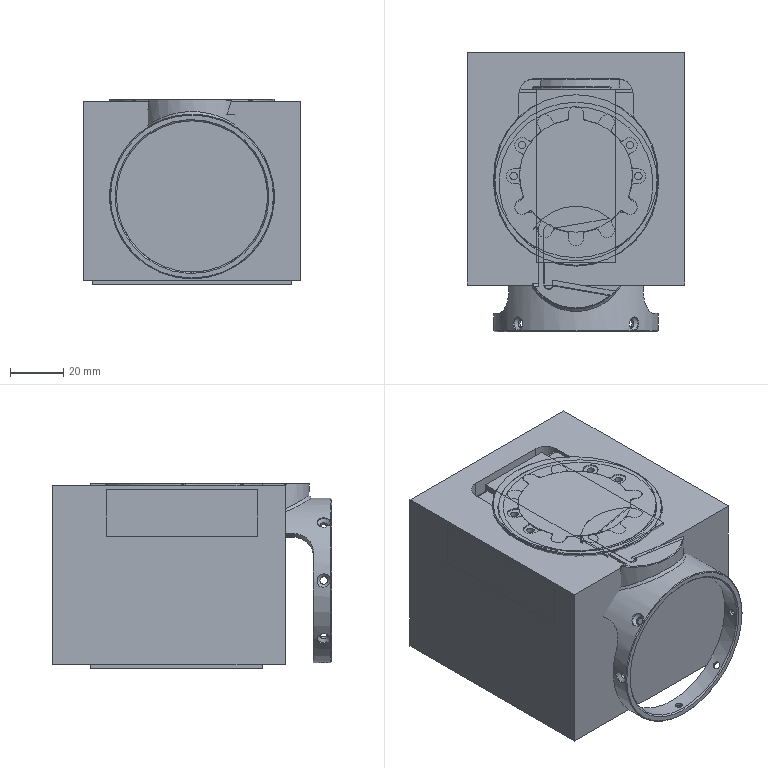NC program | NX | posted with a generic post | part box 82 x 105.2 x 70 mm
Whole program, first 1625 of 1919 lines:
N10 G17 G21 G94 G90
(轮廓开粗_2 , TOOL : 粗刀D10)
N12 T15 M6
N14 G53
N16 G17 G0 G90 X-36.218 Y-6.536 B0. C0. S7000 M3
N18 G43 Z10. H15
N20 Z2.07
N22 G94 G1 Z0.07 F2500.
N24 G41 X-32.352 Y-1.928 D15
N26 G3 X-31.65 Y0. R3.
N28 G2 X0. Y31.65 R31.65
N30 X-31.65 Y0. R-31.65
N32 G3 X-32.352 Y1.928 R3.
N34 G40
N36 G1 X-32.48 Y2.082
N38 X-29.48 Y-2.082
N40 G41 X-29.352 Y-1.928
N42 G3 X-28.65 Y0. R3.
N44 G2 X0. Y28.65 R28.65
N46 X-28.65 Y0. R-28.65
N48 G3 X-29.352 Y1.928 R3.
N50 G40
N52 G1 X-29.48 Y2.082
N54 X-26.48 Y-2.082
N56 G41 X-26.352 Y-1.928
N58 G3 X-25.65 Y0. R3.
N60 G2 X0. Y25.65 R25.65
N62 X-25.65 Y0. R-25.65
N64 G3 X-26.352 Y1.928 R3.
N66 G40
N68 G1 X-26.48 Y2.082
N70 X-23.48 Y-2.082
N72 G41 X-23.352 Y-1.928
N74 G3 X-22.65 Y0. R3.
N76 G2 X0. Y22.65 R22.65
N78 X-22.65 Y0. R-22.65
N80 G3 X-23.352 Y1.928 R3.
N82 G1 X-29.295 Y9.011
N84 G40
N86 X-29.424 Y9.165
N88 Z2.07
N90 G0 Z10.
(轮廓开粗_2_COPY , TOOL : 粗刀D10)
N92 X-1.314 Y-12.785 S5500
N94 Z-1.5
N96 G1 Z-3.5 F1500.
N98 G41 X-1.241 Y-14.137
N100 G3 X0.864 Y-16.027 R2.
N102 X16.027 Y0.864 R16.05
N104 X0.864 Y-16.027 R-16.05
N106 X2.753 Y-13.922 R2.
N108 G1 X2.691 Y-12.769
N110 G40
N112 X2.68 Y-12.57
N114 Z-1.5
N116 G0 Z10.
N118 M5
(中心孔 , TOOL : 中心钻D6)
N120 T01 M6
N122 G53
N124 G17 G0 G90 X-11.75 Y20.352 B0. C0. S2000 M3
N126 G43 Z10. H1
N128 G94 G81 G98 Z-1.5 F180. R1.
N130 X-20.352 Y11.75
N132 X-23.5 Y0.
N134 X-11.75 Y-20.352
N136 X0. Y-23.5
N138 X11.75 Y-20.352
N140 X23.5 Y0.
N142 X20.352 Y11.75
N144 X11.75 Y20.352
N146 G80
N148 G0 X11.75 Y20.352 Z10.
N150 M5
(钻头D2.9- , TOOL : 钻头D2.8)
N152 T17 M6
N154 G53
N156 G17 G0 G90 X-20.352 Y11.75 B0. C0. S2500 M3
N158 G43 Z10. H17
N160 G94 G83 G98 Z-5.341 F200. Q3. R1.
N162 X-11.75 Y20.352
N164 X11.75
N166 X20.352 Y11.75
N168 X23.5 Y0.
N170 X11.75 Y-20.352
N172 X0. Y-23.5
N174 X-11.75 Y-20.352
N176 X-23.5 Y0.
N178 G80
N180 G0 X-23.5 Y0. Z10.
N182 M5
(轮廓开粗_3 , TOOL : 粗刀D4)
N184 T18 M6
N186 G53
N188 G17 G0 G90 X4.767 Y17.977 B0. C0. S8500 M3
N190 G43 Z10. H18
N192 Z-0.329
N194 G41 G94 G1 X4.484 Y18.337 F2000. D18
N196 G3 X3.902 Y18.697 R1.
N198 G2 X0.6 Y22.76 R4.15
N200 G1 Y23.5
N202 G3 X0. Y24.1 R0.6
N204 X-0.6 Y23.5 R0.6
N206 G1 Y22.76
N208 G2 X-3.902 Y18.697 R4.15
N210 G3 X-4.484 Y18.337 R1.
N212 G1 X-4.643 Y18.134
N214 G40
N216 X-4.767 Y17.977
N218 G0 X4.767 Z-0.657
N220 G41 G1 X4.484 Y18.337
N222 G3 X3.902 Y18.697 R1.
N224 G2 X0.6 Y22.76 R4.15
N226 G1 Y23.5
N228 G3 X0. Y24.1 R0.6
N230 X-0.6 Y23.5 R0.6
N232 G1 Y22.76
N234 G2 X-3.902 Y18.697 R4.15
N236 G3 X-4.484 Y18.337 R1.
N238 G1 X-4.643 Y18.134
N240 G40
N242 X-4.767 Y17.977
N244 G0 X4.767 Z-0.986
N246 G41 G1 X4.484 Y18.337
N248 G3 X3.902 Y18.697 R1.
N250 G2 X0.6 Y22.76 R4.15
N252 G1 Y23.5
N254 G3 X0. Y24.1 R0.6
N256 X-0.6 Y23.5 R0.6
N258 G1 Y22.76
N260 G2 X-3.902 Y18.697 R4.15
N262 G3 X-4.484 Y18.337 R1.
N264 G1 X-4.643 Y18.134
N266 G40
N268 X-4.767 Y17.977
N270 G0 X4.767 Z-1.315
N272 G41 G1 X4.484 Y18.337
N274 G3 X3.902 Y18.697 R1.
N276 G2 X0.6 Y22.76 R4.15
N278 G1 Y23.5
N280 G3 X0. Y24.1 R0.6
N282 X-0.6 Y23.5 R0.6
N284 G1 Y22.76
N286 G2 X-3.902 Y18.697 R4.15
N288 G3 X-4.484 Y18.337 R1.
N290 G1 X-4.643 Y18.134
N292 G40
N294 X-4.767 Y17.977
N296 G0 X4.767 Z-1.643
N298 G41 G1 X4.484 Y18.337
N300 G3 X3.902 Y18.697 R1.
N302 G2 X0.6 Y22.76 R4.15
N304 G1 Y23.5
N306 G3 X0. Y24.1 R0.6
N308 X-0.6 Y23.5 R0.6
N310 G1 Y22.76
N312 G2 X-3.902 Y18.697 R4.15
N314 G3 X-4.484 Y18.337 R1.
N316 G1 X-4.643 Y18.134
N318 G40
N320 X-4.767 Y17.977
N322 G0 X4.767 Z-1.972
N324 G41 G1 X4.484 Y18.337
N326 G3 X3.902 Y18.697 R1.
N328 G2 X0.6 Y22.76 R4.15
N330 G1 Y23.5
N332 G3 X0. Y24.1 R0.6
N334 X-0.6 Y23.5 R0.6
N336 G1 Y22.76
N338 G2 X-3.902 Y18.697 R4.15
N340 G3 X-4.484 Y18.337 R1.
N342 G1 X-4.643 Y18.134
N344 G40
N346 X-4.767 Y17.977
N348 G0 X4.767 Z-2.301
N350 G41 G1 X4.484 Y18.337
N352 G3 X3.902 Y18.697 R1.
N354 G2 X0.6 Y22.76 R4.15
N356 G1 Y23.5
N358 G3 X0. Y24.1 R0.6
N360 X-0.6 Y23.5 R0.6
N362 G1 Y22.76
N364 G2 X-3.902 Y18.697 R4.15
N366 G3 X-4.484 Y18.337 R1.
N368 G1 X-4.643 Y18.134
N370 G40
N372 X-4.767 Y17.977
N374 G0 X4.767 Z-2.629
N376 G41 G1 X4.484 Y18.337
N378 G3 X3.902 Y18.697 R1.
N380 G2 X0.6 Y22.76 R4.15
N382 G1 Y23.5
N384 G3 X0. Y24.1 R0.6
N386 X-0.6 Y23.5 R0.6
N388 G1 Y22.76
N390 G2 X-3.902 Y18.697 R4.15
N392 G3 X-4.484 Y18.337 R1.
N394 G1 X-4.643 Y18.134
N396 G40
N398 X-4.767 Y17.977
N400 G0 X4.767 Z-2.958
N402 G41 G1 X4.484 Y18.337
N404 G3 X3.902 Y18.697 R1.
N406 G2 X0.6 Y22.76 R4.15
N408 G1 Y23.5
N410 G3 X0. Y24.1 R0.6
N412 X-0.6 Y23.5 R0.6
N414 G1 Y22.76
N416 G2 X-3.902 Y18.697 R4.15
N418 G3 X-4.484 Y18.337 R1.
N420 G1 X-4.643 Y18.134
N422 G40
N424 X-4.767 Y17.977
N426 G0 X4.767 Z-3.287
N428 G41 G1 X4.484 Y18.337
N430 G3 X3.902 Y18.697 R1.
N432 G2 X0.6 Y22.76 R4.15
N434 G1 Y23.5
N436 G3 X0. Y24.1 R0.6
N438 X-0.6 Y23.5 R0.6
N440 G1 Y22.76
N442 G2 X-3.902 Y18.697 R4.15
N444 G3 X-4.484 Y18.337 R1.
N446 G1 X-4.643 Y18.134
N448 G40
N450 X-4.767 Y17.977
N452 G0 X4.767 Z-3.615
N454 G41 G1 X4.484 Y18.337
N456 G3 X3.902 Y18.697 R1.
N458 G2 X0.6 Y22.76 R4.15
N460 G1 Y23.5
N462 G3 X0. Y24.1 R0.6
N464 X-0.6 Y23.5 R0.6
N466 G1 Y22.76
N468 G2 X-3.902 Y18.697 R4.15
N470 G3 X-4.484 Y18.337 R1.
N472 G1 X-4.643 Y18.134
N474 G40
N476 X-4.767 Y17.977
N478 G0 X4.767 Z-3.944
N480 G41 G1 X4.484 Y18.337
N482 G3 X3.902 Y18.697 R1.
N484 G2 X0.6 Y22.76 R4.15
N486 G1 Y23.5
N488 G3 X0. Y24.1 R0.6
N490 X-0.6 Y23.5 R0.6
N492 G1 Y22.76
N494 G2 X-3.902 Y18.697 R4.15
N496 G3 X-4.484 Y18.337 R1.
N498 G1 X-4.643 Y18.134
N500 G40
N502 X-4.767 Y17.977
N504 G0 X4.767 Z-4.273
N506 G41 G1 X4.484 Y18.337
N508 G3 X3.902 Y18.697 R1.
N510 G2 X0.6 Y22.76 R4.15
N512 G1 Y23.5
N514 G3 X0. Y24.1 R0.6
N516 X-0.6 Y23.5 R0.6
N518 G1 Y22.76
N520 G2 X-3.902 Y18.697 R4.15
N522 G3 X-4.484 Y18.337 R1.
N524 G1 X-4.643 Y18.134
N526 G40
N528 X-4.767 Y17.977
N530 G0 X4.767 Z-4.601
N532 G41 G1 X4.484 Y18.337
N534 G3 X3.902 Y18.697 R1.
N536 G2 X0.6 Y22.76 R4.15
N538 G1 Y23.5
N540 G3 X0. Y24.1 R0.6
N542 X-0.6 Y23.5 R0.6
N544 G1 Y22.76
N546 G2 X-3.902 Y18.697 R4.15
N548 G3 X-4.484 Y18.337 R1.
N550 G1 X-4.643 Y18.134
N552 G40
N554 X-4.767 Y17.977
N556 G0 X4.767 Z-4.93
N558 G41 G1 X4.484 Y18.337
N560 G3 X3.902 Y18.697 R1.
N562 G2 X0.6 Y22.76 R4.15
N564 G1 Y23.5
N566 G3 X0. Y24.1 R0.6
N568 X-0.6 Y23.5 R0.6
N570 G1 Y22.76
N572 G2 X-3.902 Y18.697 R4.15
N574 G3 X-4.484 Y18.337 R1.
N576 G1 X-4.643 Y18.134
N578 G40
N580 X-4.767 Y17.977
N582 G0 Z10.
N584 X-17.952 Y-4.86
N586 Z-0.329
N588 G41 G1 X-18.122 Y-5.286
N590 G3 X-18.143 Y-5.969 R1.
N592 G2 X-20.01 Y-10.86 R4.15
N594 G1 X-20.652 Y-11.23
N596 G3 X-20.871 Y-12.05 R0.6
N598 X-20.052 Y-12.27 R0.6
N600 G1 X-19.41 Y-11.899
N602 G2 X-14.241 Y-12.728 R4.15
N604 G3 X-13.638 Y-13.051 R1.
N606 G1 X-13.383 Y-13.088
N608 G40
N610 X-13.185 Y-13.117
N612 G0 X-17.952 Y-4.86 Z-0.657
N614 G41 G1 X-18.122 Y-5.286
N616 G3 X-18.143 Y-5.969 R1.
N618 G2 X-20.01 Y-10.86 R4.15
N620 G1 X-20.652 Y-11.23
N622 G3 X-20.871 Y-12.05 R0.6
N624 X-20.052 Y-12.27 R0.6
N626 G1 X-19.41 Y-11.899
N628 G2 X-14.241 Y-12.728 R4.15
N630 G3 X-13.638 Y-13.051 R1.
N632 G1 X-13.383 Y-13.088
N634 G40
N636 X-13.185 Y-13.117
N638 G0 X-17.952 Y-4.86 Z-0.986
N640 G41 G1 X-18.122 Y-5.286
N642 G3 X-18.143 Y-5.969 R1.
N644 G2 X-20.01 Y-10.86 R4.15
N646 G1 X-20.652 Y-11.23
N648 G3 X-20.871 Y-12.05 R0.6
N650 X-20.052 Y-12.27 R0.6
N652 G1 X-19.41 Y-11.899
N654 G2 X-14.241 Y-12.728 R4.15
N656 G3 X-13.638 Y-13.051 R1.
N658 G1 X-13.383 Y-13.088
N660 G40
N662 X-13.185 Y-13.117
N664 G0 X-17.952 Y-4.86 Z-1.315
N666 G41 G1 X-18.122 Y-5.286
N668 G3 X-18.143 Y-5.969 R1.
N670 G2 X-20.01 Y-10.86 R4.15
N672 G1 X-20.652 Y-11.23
N674 G3 X-20.871 Y-12.05 R0.6
N676 X-20.052 Y-12.27 R0.6
N678 G1 X-19.41 Y-11.899
N680 G2 X-14.241 Y-12.728 R4.15
N682 G3 X-13.638 Y-13.051 R1.
N684 G1 X-13.383 Y-13.088
N686 G40
N688 X-13.185 Y-13.117
N690 G0 X-17.952 Y-4.86 Z-1.643
N692 G41 G1 X-18.122 Y-5.286
N694 G3 X-18.143 Y-5.969 R1.
N696 G2 X-20.01 Y-10.86 R4.15
N698 G1 X-20.652 Y-11.23
N700 G3 X-20.871 Y-12.05 R0.6
N702 X-20.052 Y-12.27 R0.6
N704 G1 X-19.41 Y-11.899
N706 G2 X-14.241 Y-12.728 R4.15
N708 G3 X-13.638 Y-13.051 R1.
N710 G1 X-13.383 Y-13.088
N712 G40
N714 X-13.185 Y-13.117
N716 G0 X-17.952 Y-4.86 Z-1.972
N718 G41 G1 X-18.122 Y-5.286
N720 G3 X-18.143 Y-5.969 R1.
N722 G2 X-20.01 Y-10.86 R4.15
N724 G1 X-20.652 Y-11.23
N726 G3 X-20.871 Y-12.05 R0.6
N728 X-20.052 Y-12.27 R0.6
N730 G1 X-19.41 Y-11.899
N732 G2 X-14.241 Y-12.728 R4.15
N734 G3 X-13.638 Y-13.051 R1.
N736 G1 X-13.383 Y-13.088
N738 G40
N740 X-13.185 Y-13.117
N742 G0 X-17.952 Y-4.86 Z-2.301
N744 G41 G1 X-18.122 Y-5.286
N746 G3 X-18.143 Y-5.969 R1.
N748 G2 X-20.01 Y-10.86 R4.15
N750 G1 X-20.652 Y-11.23
N752 G3 X-20.871 Y-12.05 R0.6
N754 X-20.052 Y-12.27 R0.6
N756 G1 X-19.41 Y-11.899
N758 G2 X-14.241 Y-12.728 R4.15
N760 G3 X-13.638 Y-13.051 R1.
N762 G1 X-13.383 Y-13.088
N764 G40
N766 X-13.185 Y-13.117
N768 G0 X-17.952 Y-4.86 Z-2.629
N770 G41 G1 X-18.122 Y-5.286
N772 G3 X-18.143 Y-5.969 R1.
N774 G2 X-20.01 Y-10.86 R4.15
N776 G1 X-20.652 Y-11.23
N778 G3 X-20.871 Y-12.05 R0.6
N780 X-20.052 Y-12.27 R0.6
N782 G1 X-19.41 Y-11.899
N784 G2 X-14.241 Y-12.728 R4.15
N786 G3 X-13.638 Y-13.051 R1.
N788 G1 X-13.383 Y-13.088
N790 G40
N792 X-13.185 Y-13.117
N794 G0 X-17.952 Y-4.86 Z-2.958
N796 G41 G1 X-18.122 Y-5.286
N798 G3 X-18.143 Y-5.969 R1.
N800 G2 X-20.01 Y-10.86 R4.15
N802 G1 X-20.652 Y-11.23
N804 G3 X-20.871 Y-12.05 R0.6
N806 X-20.052 Y-12.27 R0.6
N808 G1 X-19.41 Y-11.899
N810 G2 X-14.241 Y-12.728 R4.15
N812 G3 X-13.638 Y-13.051 R1.
N814 G1 X-13.383 Y-13.088
N816 G40
N818 X-13.185 Y-13.117
N820 G0 X-17.952 Y-4.86 Z-3.287
N822 G41 G1 X-18.122 Y-5.286
N824 G3 X-18.143 Y-5.969 R1.
N826 G2 X-20.01 Y-10.86 R4.15
N828 G1 X-20.652 Y-11.23
N830 G3 X-20.871 Y-12.05 R0.6
N832 X-20.052 Y-12.27 R0.6
N834 G1 X-19.41 Y-11.899
N836 G2 X-14.241 Y-12.728 R4.15
N838 G3 X-13.638 Y-13.051 R1.
N840 G1 X-13.383 Y-13.088
N842 G40
N844 X-13.185 Y-13.117
N846 G0 X-17.952 Y-4.86 Z-3.615
N848 G41 G1 X-18.122 Y-5.286
N850 G3 X-18.143 Y-5.969 R1.
N852 G2 X-20.01 Y-10.86 R4.15
N854 G1 X-20.652 Y-11.23
N856 G3 X-20.871 Y-12.05 R0.6
N858 X-20.052 Y-12.27 R0.6
N860 G1 X-19.41 Y-11.899
N862 G2 X-14.241 Y-12.728 R4.15
N864 G3 X-13.638 Y-13.051 R1.
N866 G1 X-13.383 Y-13.088
N868 G40
N870 X-13.185 Y-13.117
N872 G0 X-17.952 Y-4.86 Z-3.944
N874 G41 G1 X-18.122 Y-5.286
N876 G3 X-18.143 Y-5.969 R1.
N878 G2 X-20.01 Y-10.86 R4.15
N880 G1 X-20.652 Y-11.23
N882 G3 X-20.871 Y-12.05 R0.6
N884 X-20.052 Y-12.27 R0.6
N886 G1 X-19.41 Y-11.899
N888 G2 X-14.241 Y-12.728 R4.15
N890 G3 X-13.638 Y-13.051 R1.
N892 G1 X-13.383 Y-13.088
N894 G40
N896 X-13.185 Y-13.117
N898 G0 X-17.952 Y-4.86 Z-4.273
N900 G41 G1 X-18.122 Y-5.286
N902 G3 X-18.143 Y-5.969 R1.
N904 G2 X-20.01 Y-10.86 R4.15
N906 G1 X-20.652 Y-11.23
N908 G3 X-20.871 Y-12.05 R0.6
N910 X-20.052 Y-12.27 R0.6
N912 G1 X-19.41 Y-11.899
N914 G2 X-14.241 Y-12.728 R4.15
N916 G3 X-13.638 Y-13.051 R1.
N918 G1 X-13.383 Y-13.088
N920 G40
N922 X-13.185 Y-13.117
N924 G0 X-17.952 Y-4.86 Z-4.601
N926 G41 G1 X-18.122 Y-5.286
N928 G3 X-18.143 Y-5.969 R1.
N930 G2 X-20.01 Y-10.86 R4.15
N932 G1 X-20.652 Y-11.23
N934 G3 X-20.871 Y-12.05 R0.6
N936 X-20.052 Y-12.27 R0.6
N938 G1 X-19.41 Y-11.899
N940 G2 X-14.241 Y-12.728 R4.15
N942 G3 X-13.638 Y-13.051 R1.
N944 G1 X-13.383 Y-13.088
N946 G40
N948 X-13.185 Y-13.117
N950 G0 X-17.952 Y-4.86 Z-4.93
N952 G41 G1 X-18.122 Y-5.286
N954 G3 X-18.143 Y-5.969 R1.
N956 G2 X-20.01 Y-10.86 R4.15
N958 G1 X-20.652 Y-11.23
N960 G3 X-20.871 Y-12.05 R0.6
N962 X-20.052 Y-12.27 R0.6
N964 G1 X-19.41 Y-11.899
N966 G2 X-14.241 Y-12.728 R4.15
N968 G3 X-13.638 Y-13.051 R1.
N970 G1 X-13.383 Y-13.088
N972 G40
N974 X-13.185 Y-13.117
N976 G0 Z10.
N978 X13.185
N980 Z-0.329
N982 G41 G1 X13.638 Y-13.051
N984 G3 X14.241 Y-12.728 R1.
N986 G2 X19.41 Y-11.899 R4.15
N988 G1 X20.052 Y-12.27
N990 G3 X20.871 Y-12.05 R0.6
N992 X20.652 Y-11.23 R0.6
N994 G1 X20.01 Y-10.86
N996 G2 X18.143 Y-5.969 R4.15
N998 G3 X18.122 Y-5.286 R1.
N1000 G1 X18.026 Y-5.046
N1002 G40
N1004 X17.952 Y-4.86
N1006 G0 X13.185 Y-13.117 Z-0.657
N1008 G41 G1 X13.638 Y-13.051
N1010 G3 X14.241 Y-12.728 R1.
N1012 G2 X19.41 Y-11.899 R4.15
N1014 G1 X20.052 Y-12.27
N1016 G3 X20.871 Y-12.05 R0.6
N1018 X20.652 Y-11.23 R0.6
N1020 G1 X20.01 Y-10.86
N1022 G2 X18.143 Y-5.969 R4.15
N1024 G3 X18.122 Y-5.286 R1.
N1026 G1 X18.026 Y-5.046
N1028 G40
N1030 X17.952 Y-4.86
N1032 G0 X13.185 Y-13.117 Z-0.986
N1034 G41 G1 X13.638 Y-13.051
N1036 G3 X14.241 Y-12.728 R1.
N1038 G2 X19.41 Y-11.899 R4.15
N1040 G1 X20.052 Y-12.27
N1042 G3 X20.871 Y-12.05 R0.6
N1044 X20.652 Y-11.23 R0.6
N1046 G1 X20.01 Y-10.86
N1048 G2 X18.143 Y-5.969 R4.15
N1050 G3 X18.122 Y-5.286 R1.
N1052 G1 X18.026 Y-5.046
N1054 G40
N1056 X17.952 Y-4.86
N1058 G0 X13.185 Y-13.117 Z-1.315
N1060 G41 G1 X13.638 Y-13.051
N1062 G3 X14.241 Y-12.728 R1.
N1064 G2 X19.41 Y-11.899 R4.15
N1066 G1 X20.052 Y-12.27
N1068 G3 X20.871 Y-12.05 R0.6
N1070 X20.652 Y-11.23 R0.6
N1072 G1 X20.01 Y-10.86
N1074 G2 X18.143 Y-5.969 R4.15
N1076 G3 X18.122 Y-5.286 R1.
N1078 G1 X18.026 Y-5.046
N1080 G40
N1082 X17.952 Y-4.86
N1084 G0 X13.185 Y-13.117 Z-1.643
N1086 G41 G1 X13.638 Y-13.051
N1088 G3 X14.241 Y-12.728 R1.
N1090 G2 X19.41 Y-11.899 R4.15
N1092 G1 X20.052 Y-12.27
N1094 G3 X20.871 Y-12.05 R0.6
N1096 X20.652 Y-11.23 R0.6
N1098 G1 X20.01 Y-10.86
N1100 G2 X18.143 Y-5.969 R4.15
N1102 G3 X18.122 Y-5.286 R1.
N1104 G1 X18.026 Y-5.046
N1106 G40
N1108 X17.952 Y-4.86
N1110 G0 X13.185 Y-13.117 Z-1.972
N1112 G41 G1 X13.638 Y-13.051
N1114 G3 X14.241 Y-12.728 R1.
N1116 G2 X19.41 Y-11.899 R4.15
N1118 G1 X20.052 Y-12.27
N1120 G3 X20.871 Y-12.05 R0.6
N1122 X20.652 Y-11.23 R0.6
N1124 G1 X20.01 Y-10.86
N1126 G2 X18.143 Y-5.969 R4.15
N1128 G3 X18.122 Y-5.286 R1.
N1130 G1 X18.026 Y-5.046
N1132 G40
N1134 X17.952 Y-4.86
N1136 G0 X13.185 Y-13.117 Z-2.301
N1138 G41 G1 X13.638 Y-13.051
N1140 G3 X14.241 Y-12.728 R1.
N1142 G2 X19.41 Y-11.899 R4.15
N1144 G1 X20.052 Y-12.27
N1146 G3 X20.871 Y-12.05 R0.6
N1148 X20.652 Y-11.23 R0.6
N1150 G1 X20.01 Y-10.86
N1152 G2 X18.143 Y-5.969 R4.15
N1154 G3 X18.122 Y-5.286 R1.
N1156 G1 X18.026 Y-5.046
N1158 G40
N1160 X17.952 Y-4.86
N1162 G0 X13.185 Y-13.117 Z-2.629
N1164 G41 G1 X13.638 Y-13.051
N1166 G3 X14.241 Y-12.728 R1.
N1168 G2 X19.41 Y-11.899 R4.15
N1170 G1 X20.052 Y-12.27
N1172 G3 X20.871 Y-12.05 R0.6
N1174 X20.652 Y-11.23 R0.6
N1176 G1 X20.01 Y-10.86
N1178 G2 X18.143 Y-5.969 R4.15
N1180 G3 X18.122 Y-5.286 R1.
N1182 G1 X18.026 Y-5.046
N1184 G40
N1186 X17.952 Y-4.86
N1188 G0 X13.185 Y-13.117 Z-2.958
N1190 G41 G1 X13.638 Y-13.051
N1192 G3 X14.241 Y-12.728 R1.
N1194 G2 X19.41 Y-11.899 R4.15
N1196 G1 X20.052 Y-12.27
N1198 G3 X20.871 Y-12.05 R0.6
N1200 X20.652 Y-11.23 R0.6
N1202 G1 X20.01 Y-10.86
N1204 G2 X18.143 Y-5.969 R4.15
N1206 G3 X18.122 Y-5.286 R1.
N1208 G1 X18.026 Y-5.046
N1210 G40
N1212 X17.952 Y-4.86
N1214 G0 X13.185 Y-13.117 Z-3.287
N1216 G41 G1 X13.638 Y-13.051
N1218 G3 X14.241 Y-12.728 R1.
N1220 G2 X19.41 Y-11.899 R4.15
N1222 G1 X20.052 Y-12.27
N1224 G3 X20.871 Y-12.05 R0.6
N1226 X20.652 Y-11.23 R0.6
N1228 G1 X20.01 Y-10.86
N1230 G2 X18.143 Y-5.969 R4.15
N1232 G3 X18.122 Y-5.286 R1.
N1234 G1 X18.026 Y-5.046
N1236 G40
N1238 X17.952 Y-4.86
N1240 G0 X13.185 Y-13.117 Z-3.615
N1242 G41 G1 X13.638 Y-13.051
N1244 G3 X14.241 Y-12.728 R1.
N1246 G2 X19.41 Y-11.899 R4.15
N1248 G1 X20.052 Y-12.27
N1250 G3 X20.871 Y-12.05 R0.6
N1252 X20.652 Y-11.23 R0.6
N1254 G1 X20.01 Y-10.86
N1256 G2 X18.143 Y-5.969 R4.15
N1258 G3 X18.122 Y-5.286 R1.
N1260 G1 X18.026 Y-5.046
N1262 G40
N1264 X17.952 Y-4.86
N1266 G0 X13.185 Y-13.117 Z-3.944
N1268 G41 G1 X13.638 Y-13.051
N1270 G3 X14.241 Y-12.728 R1.
N1272 G2 X19.41 Y-11.899 R4.15
N1274 G1 X20.052 Y-12.27
N1276 G3 X20.871 Y-12.05 R0.6
N1278 X20.652 Y-11.23 R0.6
N1280 G1 X20.01 Y-10.86
N1282 G2 X18.143 Y-5.969 R4.15
N1284 G3 X18.122 Y-5.286 R1.
N1286 G1 X18.026 Y-5.046
N1288 G40
N1290 X17.952 Y-4.86
N1292 G0 X13.185 Y-13.117 Z-4.273
N1294 G41 G1 X13.638 Y-13.051
N1296 G3 X14.241 Y-12.728 R1.
N1298 G2 X19.41 Y-11.899 R4.15
N1300 G1 X20.052 Y-12.27
N1302 G3 X20.871 Y-12.05 R0.6
N1304 X20.652 Y-11.23 R0.6
N1306 G1 X20.01 Y-10.86
N1308 G2 X18.143 Y-5.969 R4.15
N1310 G3 X18.122 Y-5.286 R1.
N1312 G1 X18.026 Y-5.046
N1314 G40
N1316 X17.952 Y-4.86
N1318 G0 X13.185 Y-13.117 Z-4.601
N1320 G41 G1 X13.638 Y-13.051
N1322 G3 X14.241 Y-12.728 R1.
N1324 G2 X19.41 Y-11.899 R4.15
N1326 G1 X20.052 Y-12.27
N1328 G3 X20.871 Y-12.05 R0.6
N1330 X20.652 Y-11.23 R0.6
N1332 G1 X20.01 Y-10.86
N1334 G2 X18.143 Y-5.969 R4.15
N1336 G3 X18.122 Y-5.286 R1.
N1338 G1 X18.026 Y-5.046
N1340 G40
N1342 X17.952 Y-4.86
N1344 G0 X13.185 Y-13.117 Z-4.93
N1346 G41 G1 X13.638 Y-13.051
N1348 G3 X14.241 Y-12.728 R1.
N1350 G2 X19.41 Y-11.899 R4.15
N1352 G1 X20.052 Y-12.27
N1354 G3 X20.871 Y-12.05 R0.6
N1356 X20.652 Y-11.23 R0.6
N1358 G1 X20.01 Y-10.86
N1360 G2 X18.143 Y-5.969 R4.15
N1362 G3 X18.122 Y-5.286 R1.
N1364 G1 X18.026 Y-5.046
N1366 G40
N1368 X17.952 Y-4.86
N1370 G0 Z10.
(轮廓开粗_3_COPY , TOOL : 粗刀D4)
N1372 X-17.728 Y5.559
N1374 Z-0.215
N1376 G41 G1 X-18.125 Y5.274
N1378 G3 X-18.511 Y4.708 R1.
N1380 X-18.827 Y3.219 R19.1
N1382 G2 X-21.932 Y0.6 R3.15
N1384 G1 X-23.5
N1386 G3 X-24.1 Y0. R0.6
N1388 X-23.5 Y-0.6 R0.6
N1390 G1 X-21.932
N1392 G2 X-18.827 Y-3.219 R3.15
N1394 G3 X-18.143 Y-5.969 R19.1
N1396 G2 X-20.01 Y-10.86 R4.15
N1398 G1 X-20.652 Y-11.23
N1400 G3 X-20.871 Y-12.05 R0.6
N1402 X-20.052 Y-12.27 R0.6
N1404 G1 X-19.41 Y-11.899
N1406 G2 X-14.241 Y-12.728 R4.15
N1408 G3 X-12.201 Y-14.695 R19.1
N1410 G2 X-11.485 Y-18.693 R3.15
N1412 G1 X-12.27 Y-20.052
N1414 G3 X-12.05 Y-20.871 R0.6
N1416 X-11.23 Y-20.652 R0.6
N1418 G1 X-10.446 Y-19.293
N1420 G2 X-6.626 Y-17.914 R3.15
N1422 G3 X-3.219 Y-18.827 R19.1
N1424 G2 X-0.6 Y-21.932 R3.15
N1426 G1 Y-23.5
N1428 G3 X0. Y-24.1 R0.6
N1430 X0.6 Y-23.5 R0.6
N1432 G1 Y-21.932
N1434 G2 X3.219 Y-18.827 R3.15
N1436 G3 X6.626 Y-17.914 R19.1
N1438 G2 X10.446 Y-19.293 R3.15
N1440 G1 X11.23 Y-20.652
N1442 G3 X12.05 Y-20.871 R0.6
N1444 X12.27 Y-20.052 R0.6
N1446 G1 X11.485 Y-18.693
N1448 G2 X12.201 Y-14.695 R3.15
N1450 G3 X14.241 Y-12.728 R19.1
N1452 G2 X19.41 Y-11.899 R4.15
N1454 G1 X20.052 Y-12.27
N1456 G3 X20.871 Y-12.05 R0.6
N1458 X20.652 Y-11.23 R0.6
N1460 G1 X20.01 Y-10.86
N1462 G2 X18.143 Y-5.969 R4.15
N1464 G3 X18.827 Y-3.219 R19.1
N1466 G2 X21.932 Y-0.6 R3.15
N1468 G1 X23.5
N1470 G3 X24.1 Y0. R0.6
N1472 X23.5 Y0.6 R0.6
N1474 G1 X21.932
N1476 G2 X18.827 Y3.219 R3.15
N1478 G3 X17.914 Y6.626 R19.1
N1480 G2 X19.293 Y10.446 R3.15
N1482 G1 X20.652 Y11.23
N1484 G3 X20.871 Y12.05 R0.6
N1486 X20.052 Y12.27 R0.6
N1488 G1 X18.693 Y11.485
N1490 G2 X14.695 Y12.201 R3.15
N1492 G3 X12.201 Y14.695 R19.1
N1494 G2 X11.485 Y18.693 R3.15
N1496 G1 X12.27 Y20.052
N1498 G3 X12.05 Y20.871 R0.6
N1500 X11.23 Y20.652 R0.6
N1502 G1 X10.446 Y19.293
N1504 G2 X6.626 Y17.914 R3.15
N1506 G3 X3.902 Y18.697 R19.1
N1508 G2 X0.6 Y22.76 R4.15
N1510 G1 Y23.5
N1512 G3 X0. Y24.1 R0.6
N1514 X-0.6 Y23.5 R0.6
N1516 G1 Y22.76
N1518 G2 X-3.902 Y18.697 R4.15
N1520 G3 X-6.626 Y17.914 R19.1
N1522 G2 X-10.446 Y19.293 R3.15
N1524 G1 X-11.23 Y20.652
N1526 G3 X-12.05 Y20.871 R0.6
N1528 X-12.27 Y20.052 R0.6
N1530 G1 X-11.485 Y18.693
N1532 G2 X-12.201 Y14.695 R3.15
N1534 G3 X-14.695 Y12.201 R19.1
N1536 G2 X-18.693 Y11.485 R3.15
N1538 G1 X-20.052 Y12.27
N1540 G3 X-20.871 Y12.05 R0.6
N1542 X-20.652 Y11.23 R0.6
N1544 G1 X-19.293 Y10.446
N1546 G2 X-17.914 Y6.626 R3.15
N1548 G3 X-18.511 Y4.708 R19.1
N1550 X-18.442 Y4.028 R1.
N1552 G1 X-18.317 Y3.767
N1554 G40
N1556 X-18.23 Y3.587
N1558 G0 X-17.728 Y5.559 Z-0.43
N1560 G41 G1 X-18.125 Y5.274
N1562 G3 X-18.511 Y4.708 R1.
N1564 X-18.827 Y3.219 R19.1
N1566 G2 X-21.932 Y0.6 R3.15
N1568 G1 X-23.5
N1570 G3 X-24.1 Y0. R0.6
N1572 X-23.5 Y-0.6 R0.6
N1574 G1 X-21.932
N1576 G2 X-18.827 Y-3.219 R3.15
N1578 G3 X-18.143 Y-5.969 R19.1
N1580 G2 X-20.01 Y-10.86 R4.15
N1582 G1 X-20.652 Y-11.23
N1584 G3 X-20.871 Y-12.05 R0.6
N1586 X-20.052 Y-12.27 R0.6
N1588 G1 X-19.41 Y-11.899
N1590 G2 X-14.241 Y-12.728 R4.15
N1592 G3 X-12.201 Y-14.695 R19.1
N1594 G2 X-11.485 Y-18.693 R3.15
N1596 G1 X-12.27 Y-20.052
N1598 G3 X-12.05 Y-20.871 R0.6
N1600 X-11.23 Y-20.652 R0.6
N1602 G1 X-10.446 Y-19.293
N1604 G2 X-6.626 Y-17.914 R3.15
N1606 G3 X-3.219 Y-18.827 R19.1
N1608 G2 X-0.6 Y-21.932 R3.15
N1610 G1 Y-23.5
N1612 G3 X0. Y-24.1 R0.6
N1614 X0.6 Y-23.5 R0.6
N1616 G1 Y-21.932
N1618 G2 X3.219 Y-18.827 R3.15
N1620 G3 X6.626 Y-17.914 R19.1
N1622 G2 X10.446 Y-19.293 R3.15
N1624 G1 X11.23 Y-20.652
N1626 G3 X12.05 Y-20.871 R0.6
N1628 X12.27 Y-20.052 R0.6
N1630 G1 X11.485 Y-18.693
N1632 G2 X12.201 Y-14.695 R3.15
N1634 G3 X14.241 Y-12.728 R19.1
N1636 G2 X19.41 Y-11.899 R4.15
N1638 G1 X20.052 Y-12.27
N1640 G3 X20.871 Y-12.05 R0.6
N1642 X20.652 Y-11.23 R0.6
N1644 G1 X20.01 Y-10.86
N1646 G2 X18.143 Y-5.969 R4.15
N1648 G3 X18.827 Y-3.219 R19.1
N1650 G2 X21.932 Y-0.6 R3.15
N1652 G1 X23.5
N1654 G3 X24.1 Y0. R0.6
N1656 X23.5 Y0.6 R0.6
N1658 G1 X21.932
N1660 G2 X18.827 Y3.219 R3.15
N1662 G3 X17.914 Y6.626 R19.1
N1664 G2 X19.293 Y10.446 R3.15
N1666 G1 X20.652 Y11.23
N1668 G3 X20.871 Y12.05 R0.6
N1670 X20.052 Y12.27 R0.6
N1672 G1 X18.693 Y11.485
N1674 G2 X14.695 Y12.201 R3.15
N1676 G3 X12.201 Y14.695 R19.1
N1678 G2 X11.485 Y18.693 R3.15
N1680 G1 X12.27 Y20.052
N1682 G3 X12.05 Y20.871 R0.6
N1684 X11.23 Y20.652 R0.6
N1686 G1 X10.446 Y19.293
N1688 G2 X6.626 Y17.914 R3.15
N1690 G3 X3.902 Y18.697 R19.1
N1692 G2 X0.6 Y22.76 R4.15
N1694 G1 Y23.5
N1696 G3 X0. Y24.1 R0.6
N1698 X-0.6 Y23.5 R0.6
N1700 G1 Y22.76
N1702 G2 X-3.902 Y18.697 R4.15
N1704 G3 X-6.626 Y17.914 R19.1
N1706 G2 X-10.446 Y19.293 R3.15
N1708 G1 X-11.23 Y20.652
N1710 G3 X-12.05 Y20.871 R0.6
N1712 X-12.27 Y20.052 R0.6
N1714 G1 X-11.485 Y18.693
N1716 G2 X-12.201 Y14.695 R3.15
N1718 G3 X-14.695 Y12.201 R19.1
N1720 G2 X-18.693 Y11.485 R3.15
N1722 G1 X-20.052 Y12.27
N1724 G3 X-20.871 Y12.05 R0.6
N1726 X-20.652 Y11.23 R0.6
N1728 G1 X-19.293 Y10.446
N1730 G2 X-17.914 Y6.626 R3.15
N1732 G3 X-18.511 Y4.708 R19.1
N1734 X-18.442 Y4.028 R1.
N1736 G1 X-18.317 Y3.767
N1738 G40
N1740 X-18.23 Y3.587
N1742 G0 Z10.
N1744 M5
(单向轮廓精光_8 , TOOL : 光刀D10)
N1746 T10 M6
N1748 G53
N1750 G17 G0 G90 X-11.787 Y-5.603 B0. C0. S8000 M3
N1752 G43 Z10. H10
N1754 Z-2.
N1756 G94 G1 Z-5. F1200.
N1758 G41 X-13.728 Y-6.716 D10
N1760 G3 X-14.098 Y-8.081 R1.
N1762 X8.081 Y-14.098 R16.25
N1764 X-14.098 Y-8.081 R-16.25
N1766 X-13.843 Y-8.51 R16.25
N1768 X-12.468 Y-8.839 R1.
N1770 G1 X-10.732 Y-7.771
N1772 G40
N1774 X-10.561 Y-7.667
N1776 Z-2.
N1778 G0 Z10.
(单向轮廓精光_8_COPY , TOOL : 光刀D10)
N1780 X-31.549 Y-19.235 S7000
N1782 Z3.
N1784 G1 Z0.
N1786 G41 X-26.181 Y-16.158
N1788 G3 X-25.811 Y-14.794 R1.
N1790 G2 X-14.794 Y25.811 R29.75
N1792 X-25.811 Y-14.794 R-29.75
N1794 X-26.056 Y-14.358 R29.75
N1796 G3 X-27.415 Y-13.964 R1.
N1798 G40
N1800 G1 X-27.59 Y-14.061
N1802 X-22.451 Y-14.02
N1804 G41 X-22.277 Y-13.921
N1806 G3 X-21.907 Y-12.556 R1.
N1808 G2 X-12.556 Y21.907 R25.25
N1810 X-21.907 Y-12.556 R-25.25
N1812 X-22.151 Y-12.12 R25.25
N1814 G3 X-23.508 Y-11.722 R1.
N1816 G1 X-32.708 Y-16.756
N1818 G40
N1820 X-32.883 Y-16.852
N1822 Z3.
N1824 G0 Z10.
N1826 M5
(单向轮廓精光_9 , TOOL : 光刀D4)
N1828 T07 M6
N1830 G53
N1832 G17 G0 G90 X-5.251 Y17.079 B0. C0. S8000 M3
N1834 G43 Z10. H7
N1836 Z2.5
N1838 G94 G1 Z-0.5 F1200.
N1840 G41 X-5.389 Y17.454 D7
N1842 G3 X-6.674 Y18.045 R1.
N1844 G2 X-10.325 Y19.363 R3.01
N1846 G1 X-11.109 Y20.722
N1848 G3 X-12.12 Y20.992 R0.74
N1850 X-12.391 Y19.982 R0.74
N1852 G1 X-11.607 Y18.623
N1854 G2 X-12.291 Y14.803 R3.01
N1856 G3 X-12.421 Y13.394 R1.
N1858 G1 X-12.293 Y13.241
N1860 G40
N1862 X-12.166 Y13.087
N1864 Z2.5
N1866 G0 Z10.
N1868 X-5.251 Y17.079
N1870 Z2.5
N1872 G1 Z-0.5
N1874 G41 X-5.396 Y17.473
N1876 G3 X-6.681 Y18.064 R1.
N1878 G2 X-10.308 Y19.373 R2.99
N1880 G1 X-11.092 Y20.732
N1882 G3 X-12.13 Y21.01 R0.76
N1884 X-12.408 Y19.972 R0.76
N1886 G1 X-11.624 Y18.613
N1888 G2 X-12.303 Y14.818 R2.99
N1890 G3 X-12.434 Y13.41 R1.
N1892 G1 X-12.293 Y13.241
N1894 G40
N1896 X-12.166 Y13.087
N1898 Z2.5
N1900 G0 Z10.
N1902 X-13.087 Y12.166
N1904 Z2.5
N1906 G1 Z-0.5
N1908 G41 X-13.394 Y12.421
N1910 G3 X-14.803 Y12.291 R1.
N1912 G2 X-18.623 Y11.607 R3.01
N1914 G1 X-19.982 Y12.391
N1916 G3 X-20.992 Y12.12 R0.74
N1918 X-20.722 Y11.109 R0.74
N1920 G1 X-19.363 Y10.325
N1922 G2 X-18.045 Y6.674 R3.01
N1924 G3 X-17.454 Y5.389 R1.
N1926 G1 X-17.267 Y5.32
N1928 G40
N1930 X-17.079 Y5.251
N1932 Z2.5
N1934 G0 Z10.
N1936 X-13.087 Y12.166
N1938 Z2.5
N1940 G1 Z-0.5
N1942 G41 X-13.41 Y12.434
N1944 G3 X-14.818 Y12.303 R1.
N1946 G2 X-18.613 Y11.624 R2.99
N1948 G1 X-19.972 Y12.408
N1950 G3 X-21.01 Y12.13 R0.76
N1952 X-20.732 Y11.092 R0.76
N1954 G1 X-19.373 Y10.308
N1956 G2 X-18.064 Y6.681 R2.99
N1958 G3 X-17.473 Y5.396 R1.
N1960 G1 X-17.267 Y5.32
N1962 G40
N1964 X-17.079 Y5.251
N1966 Z2.5
N1968 G0 Z10.
N1970 X-17.416 Y3.992
N1972 Z2.5
N1974 G1 Z-0.5
N1976 G41 X-17.811 Y4.06
N1978 G3 X-18.965 Y3.243 R1.
N1980 G2 X-21.932 Y0.74 R3.01
N1982 G1 X-23.5
N1984 G3 X-24.24 Y0. R0.74
N1986 X-23.5 Y-0.74 R0.74
N1988 G1 X-21.932
N1990 G2 X-18.965 Y-3.243 R3.01
N1992 G3 X-17.811 Y-4.06 R1.
N1994 G1 X-17.613 Y-4.026
N1996 G40
N1998 X-17.416 Y-3.992
N2000 Z2.5
N2002 G0 Z10.
N2004 Y3.992
N2006 Z2.5
N2008 G1 Z-0.5
N2010 G41 X-17.83 Y4.063
N2012 G3 X-18.984 Y3.246 R1.
N2014 G2 X-21.932 Y0.76 R2.99
N2016 G1 X-23.5
N2018 G3 X-24.26 Y0. R0.76
N2020 X-23.5 Y-0.76 R0.76
N2022 G1 X-21.932
N2024 G2 X-18.984 Y-3.246 R2.99
N2026 G3 X-17.83 Y-4.063 R1.
N2028 G1 X-17.613 Y-4.026
N2030 G40
N2032 X-17.416 Y-3.992
N2034 Z2.5
N2036 G0 Z10.
N2038 X-12.166 Y-13.087
N2040 Z2.5
N2042 G1 Z-0.5
N2044 G41 X-12.421 Y-13.394
N2046 G3 X-12.291 Y-14.803 R1.
N2048 G2 X-11.607 Y-18.623 R3.01
N2050 G1 X-12.391 Y-19.982
N2052 G3 X-12.12 Y-20.992 R0.74
N2054 X-11.109 Y-20.722 R0.74
N2056 G1 X-10.325 Y-19.363
N2058 G2 X-6.674 Y-18.045 R3.01
N2060 G3 X-5.389 Y-17.454 R1.
N2062 G1 X-5.32 Y-17.267
N2064 G40
N2066 X-5.251 Y-17.079
N2068 Z2.5
N2070 G0 Z10.
N2072 X-12.166 Y-13.087
N2074 Z2.5
N2076 G1 Z-0.5
N2078 G41 X-12.434 Y-13.41
N2080 G3 X-12.303 Y-14.818 R1.
N2082 G2 X-11.624 Y-18.613 R2.99
N2084 G1 X-12.408 Y-19.972
N2086 G3 X-12.13 Y-21.01 R0.76
N2088 X-11.092 Y-20.732 R0.76
N2090 G1 X-10.308 Y-19.373
N2092 G2 X-6.681 Y-18.064 R2.99
N2094 G3 X-5.396 Y-17.473 R1.
N2096 G1 X-5.32 Y-17.267
N2098 G40
N2100 X-5.251 Y-17.079
N2102 Z2.5
N2104 G0 Z10.
N2106 X-3.992 Y-17.416
N2108 Z2.5
N2110 G1 Z-0.5
N2112 G41 X-4.06 Y-17.811
N2114 G3 X-3.243 Y-18.965 R1.
N2116 G2 X-0.74 Y-21.932 R3.01
N2118 G1 Y-23.5
N2120 G3 X0. Y-24.24 R0.74
N2122 X0.74 Y-23.5 R0.74
N2124 G1 Y-21.932
N2126 G2 X3.243 Y-18.965 R3.01
N2128 G3 X4.06 Y-17.811 R1.
N2130 G1 X4.026 Y-17.613
N2132 G40
N2134 X3.992 Y-17.416
N2136 Z2.5
N2138 G0 Z10.
N2140 X-3.992
N2142 Z2.5
N2144 G1 Z-0.5
N2146 G41 X-4.063 Y-17.83
N2148 G3 X-3.246 Y-18.984 R1.
N2150 G2 X-0.76 Y-21.932 R2.99
N2152 G1 Y-23.5
N2154 G3 X0. Y-24.26 R0.76
N2156 X0.76 Y-23.5 R0.76
N2158 G1 Y-21.932
N2160 G2 X3.246 Y-18.984 R2.99
N2162 G3 X4.063 Y-17.83 R1.
N2164 G1 X4.026 Y-17.613
N2166 G40
N2168 X3.992 Y-17.416
N2170 Z2.5
N2172 G0 Z10.
N2174 X5.251 Y-17.079
N2176 Z2.5
N2178 G1 Z-0.5
N2180 G41 X5.389 Y-17.454
N2182 G3 X6.674 Y-18.045 R1.
N2184 G2 X10.325 Y-19.363 R3.01
N2186 G1 X11.109 Y-20.722
N2188 G3 X12.12 Y-20.992 R0.74
N2190 X12.391 Y-19.982 R0.74
N2192 G1 X11.607 Y-18.623
N2194 G2 X12.291 Y-14.803 R3.01
N2196 G3 X12.421 Y-13.394 R1.
N2198 G1 X12.293 Y-13.241
N2200 G40
N2202 X12.166 Y-13.087
N2204 Z2.5
N2206 G0 Z10.
N2208 X5.251 Y-17.079
N2210 Z2.5
N2212 G1 Z-0.5
N2214 G41 X5.396 Y-17.473
N2216 G3 X6.681 Y-18.064 R1.
N2218 G2 X10.308 Y-19.373 R2.99
N2220 G1 X11.092 Y-20.732
N2222 G3 X12.13 Y-21.01 R0.76
N2224 X12.408 Y-19.972 R0.76
N2226 G1 X11.624 Y-18.613
N2228 G2 X12.303 Y-14.818 R2.99
N2230 G3 X12.434 Y-13.41 R1.
N2232 G1 X12.293 Y-13.241
N2234 G40
N2236 X12.166 Y-13.087
N2238 Z2.5
N2240 G0 Z10.
N2242 X17.416 Y-3.992
N2244 Z2.5
N2246 G1 Z-0.5
N2248 G41 X17.811 Y-4.06
N2250 G3 X18.965 Y-3.243 R1.
N2252 G2 X21.932 Y-0.74 R3.01
N2254 G1 X23.5
N2256 G3 X24.24 Y0. R0.74
N2258 X23.5 Y0.74 R0.74
N2260 G1 X21.932
N2262 G2 X18.965 Y3.243 R3.01
N2264 G3 X17.811 Y4.06 R1.
N2266 G1 X17.613 Y4.026
N2268 G40
N2270 X17.416 Y3.992
N2272 Z2.5
N2274 G0 Z10.
N2276 Y-3.992
N2278 Z2.5
N2280 G1 Z-0.5
N2282 G41 X17.83 Y-4.063
N2284 G3 X18.984 Y-3.246 R1.
N2286 G2 X21.932 Y-0.76 R2.99
N2288 G1 X23.5
N2290 G3 X24.26 Y0. R0.76
N2292 X23.5 Y0.76 R0.76
N2294 G1 X21.932
N2296 G2 X18.984 Y3.246 R2.99
N2298 G3 X17.83 Y4.063 R1.
N2300 G1 X17.613 Y4.026
N2302 G40
N2304 X17.416 Y3.992
N2306 Z2.5
N2308 G0 Z10.
N2310 X17.079 Y5.251
N2312 Z2.5
N2314 G1 Z-0.5
N2316 G41 X17.454 Y5.389
N2318 G3 X18.045 Y6.674 R1.
N2320 G2 X19.363 Y10.325 R3.01
N2322 G1 X20.722 Y11.109
N2324 G3 X20.992 Y12.12 R0.74
N2326 X19.982 Y12.391 R0.74
N2328 G1 X18.623 Y11.607
N2330 G2 X14.803 Y12.291 R3.01
N2332 G3 X13.394 Y12.421 R1.
N2334 G1 X13.241 Y12.293
N2336 G40
N2338 X13.087 Y12.166
N2340 Z2.5
N2342 G0 Z10.
N2344 X17.079 Y5.251
N2346 Z2.5
N2348 G1 Z-0.5
N2350 G41 X17.473 Y5.396
N2352 G3 X18.064 Y6.681 R1.
N2354 G2 X19.373 Y10.308 R2.99
N2356 G1 X20.732 Y11.092
N2358 G3 X21.01 Y12.13 R0.76
N2360 X19.972 Y12.408 R0.76
N2362 G1 X18.613 Y11.624
N2364 G2 X14.818 Y12.303 R2.99
N2366 G3 X13.41 Y12.434 R1.
N2368 G1 X13.241 Y12.293
N2370 G40
N2372 X13.087 Y12.166
N2374 Z2.5
N2376 G0 Z10.
N2378 X12.166 Y13.087
N2380 Z2.5
N2382 G1 Z-0.5
N2384 G41 X12.421 Y13.394
N2386 G3 X12.291 Y14.803 R1.
N2388 G2 X11.607 Y18.623 R3.01
N2390 G1 X12.391 Y19.982
N2392 G3 X12.12 Y20.992 R0.74
N2394 X11.109 Y20.722 R0.74
N2396 G1 X10.325 Y19.363
N2398 G2 X6.674 Y18.045 R3.01
N2400 G3 X5.389 Y17.454 R1.
N2402 G1 X5.32 Y17.267
N2404 G40
N2406 X5.251 Y17.079
N2408 Z2.5
N2410 G0 Z10.
N2412 X12.166 Y13.087
N2414 Z2.5
N2416 G1 Z-0.5
N2418 G41 X12.434 Y13.41
N2420 G3 X12.303 Y14.818 R1.
N2422 G2 X11.624 Y18.613 R2.99
N2424 G1 X12.408 Y19.972
N2426 G3 X12.13 Y21.01 R0.76
N2428 X11.092 Y20.732 R0.76
N2430 G1 X10.308 Y19.373
N2432 G2 X6.681 Y18.064 R2.99
N2434 G3 X5.396 Y17.473 R1.
N2436 G1 X5.32 Y17.267
N2438 G40
N2440 X5.251 Y17.079
N2442 Z2.5
N2444 G0 Z10.
(单向轮廓精光_9_COPY , TOOL : 光刀D4)
N2446 X0.026 Y20.458
N2448 Z-2.
N2450 G1 Z-5.
N2452 G41 X-0.245 Y22.5
N2454 G3 X0.755 Y23.5 R1.
N2456 X0. Y24.255 R0.755
N2458 X-0.755 Y23.5 R0.755
N2460 G1 Y22.76
N2462 G2 X-3.934 Y18.849 R3.995
N2464 G3 X-18.291 Y-6.018 R19.255
N2466 G2 X-20.088 Y-10.726 R3.995
N2468 G1 X-20.729 Y-11.096
N2470 G3 X-21.005 Y-12.128 R0.755
N2472 X-19.974 Y-12.404 R0.755
N2474 G1 X-19.333 Y-12.034
N2476 G2 X-14.357 Y-12.831 R3.995
N2478 G3 X14.357 Y-12.831 R19.255
N2480 G2 X19.333 Y-12.034 R3.995
N2482 G1 X19.974 Y-12.404
N2484 G3 X21.005 Y-12.128 R0.755
N2486 X20.729 Y-11.096 R0.755
N2488 G1 X20.088 Y-10.726
N2490 G2 X18.291 Y-6.018 R3.995
N2492 G3 X3.934 Y18.849 R19.255
N2494 G2 X0.755 Y22.76 R3.995
N2496 G1 Y23.5
N2498 G3 X0.595 Y23.964 R0.755
N2500 X-0.106 Y24.051 R0.5
N2502 G40
N2504 G1 X-0.264 Y23.928
N2506 X-0.425 Y22.5
N2508 G41 X-0.225
N2510 G3 X0.775 Y23.5 R1.
N2512 X0. Y24.275 R0.775
N2514 X-0.775 Y23.5 R0.775
N2516 G1 Y22.76
N2518 G2 X-3.938 Y18.868 R3.975
N2520 G3 X-18.31 Y-6.024 R19.275
N2522 G2 X-20.098 Y-10.709 R3.975
N2524 G1 X-20.739 Y-11.079
N2526 G3 X-21.023 Y-12.138 R0.775
N2528 X-19.964 Y-12.421 R0.775
N2530 G1 X-19.323 Y-12.051
N2532 G2 X-14.372 Y-12.845 R3.975
N2534 G3 X14.372 Y-12.845 R19.275
N2536 G2 X19.323 Y-12.051 R3.975
N2538 G1 X19.964 Y-12.421
N2540 G3 X21.023 Y-12.138 R0.775
N2542 X20.739 Y-11.079 R0.775
N2544 G1 X20.098 Y-10.709
N2546 G2 X18.31 Y-6.024 R3.975
N2548 G3 X3.938 Y18.868 R19.275
N2550 G2 X0.775 Y22.76 R3.975
N2552 G1 Y23.5
N2554 G3 X0.619 Y23.966 R0.775
N2556 X-0.081 Y24.065 R0.5
N2558 G40
N2560 G1 X0. Y20.706
N2562 Z-2.
N2564 G0 Z10.
N2566 M5
(倒角刀D6._2 , TOOL : 倒角刀D4)
N2568 T11 M6
N2570 G53
N2572 G17 G0 G90 X-19.115 Y5.536 B0. C0. S7500 M3
N2574 G43 Z10. H11
N2576 Z2.55
N2578 G94 G1 Z-0.45 F1200.
N2580 G41 X-19.698 Y5.692 D11
N2582 G3 X-20.188 Y5.409 R0.4
N2584 X-20.601 Y3.522 R20.9
N2586 G2 X-21.932 Y2.4 R1.35
N2588 G1 X-23.5
N2590 G3 X-25.9 Y0. R2.4
N2592 X-23.5 Y-2.4 R2.4
N2594 G1 X-21.932
N2596 G2 X-20.601 Y-3.522 R1.35
N2598 G3 X-19.853 Y-6.532 R20.9
N2600 G2 X-20.91 Y-9.301 R2.35
N2602 G1 X-21.552 Y-9.672
N2604 G3 X-22.43 Y-12.95 R2.4
N2606 X-19.152 Y-13.828 R2.4
N2608 G1 X-18.51 Y-13.458
N2610 G2 X-15.583 Y-13.927 R2.35
N2612 G3 X-13.351 Y-16.08 R20.9
N2614 G2 X-13.044 Y-17.793 R1.35
N2616 G1 X-13.828 Y-19.152
N2618 G3 X-12.95 Y-22.43 R2.4
N2620 X-9.672 Y-21.552 R2.4
N2622 G1 X-8.887 Y-20.193
N2624 G2 X-7.25 Y-19.602 R1.35
N2626 G3 X-3.522 Y-20.601 R20.9
N2628 G2 X-2.4 Y-21.932 R1.35
N2630 G1 Y-23.5
N2632 G3 X0. Y-25.9 R2.4
N2634 X2.4 Y-23.5 R2.4
N2636 G1 Y-21.932
N2638 G2 X3.522 Y-20.601 R1.35
N2640 G3 X7.25 Y-19.602 R20.9
N2642 G2 X8.887 Y-20.193 R1.35
N2644 G1 X9.672 Y-21.552
N2646 G3 X12.95 Y-22.43 R2.4
N2648 X13.828 Y-19.152 R2.4
N2650 G1 X13.044 Y-17.793
N2652 G2 X13.351 Y-16.08 R1.35
N2654 G3 X15.583 Y-13.927 R20.9
N2656 G2 X18.51 Y-13.458 R2.35
N2658 G1 X19.152 Y-13.828
N2660 G3 X22.43 Y-12.95 R2.4
N2662 X21.552 Y-9.672 R2.4
N2664 G1 X20.91 Y-9.301
N2666 G2 X19.853 Y-6.532 R2.35
N2668 G3 X20.601 Y-3.522 R20.9
N2670 G2 X21.932 Y-2.4 R1.35
N2672 G1 X23.5
N2674 G3 X25.9 Y0. R2.4
N2676 X23.5 Y2.4 R2.4
N2678 G1 X21.932
N2680 G2 X20.601 Y3.522 R1.35
N2682 G3 X19.602 Y7.25 R20.9
N2684 G2 X20.193 Y8.887 R1.35
N2686 G1 X21.552 Y9.672
N2688 G3 X22.43 Y12.95 R2.4
N2690 X19.152 Y13.828 R2.4
N2692 G1 X17.793 Y13.044
N2694 G2 X16.08 Y13.351 R1.35
N2696 G3 X13.351 Y16.08 R20.9
N2698 G2 X13.044 Y17.793 R1.35
N2700 G1 X13.828 Y19.152
N2702 G3 X12.95 Y22.43 R2.4
N2704 X9.672 Y21.552 R2.4
N2706 G1 X8.887 Y20.193
N2708 G2 X7.25 Y19.602 R1.35
N2710 G3 X4.27 Y20.459 R20.9
N2712 G2 X2.4 Y22.76 R2.35
N2714 G1 Y23.5
N2716 G3 X0. Y25.9 R2.4
N2718 X-2.4 Y23.5 R2.4
N2720 G1 Y22.76
N2722 G2 X-4.27 Y20.459 R2.35
N2724 G3 X-7.25 Y19.602 R20.9
N2726 G2 X-8.887 Y20.193 R1.35
N2728 G1 X-9.672 Y21.552
N2730 G3 X-12.95 Y22.43 R2.4
N2732 X-13.828 Y19.152 R2.4
N2734 G1 X-13.044 Y17.793
N2736 G2 X-13.351 Y16.08 R1.35
N2738 G3 X-16.08 Y13.351 R20.9
N2740 G2 X-17.793 Y13.044 R1.35
N2742 G1 X-19.152 Y13.828
N2744 G3 X-22.43 Y12.95 R2.4
N2746 X-21.552 Y9.672 R2.4
N2748 G1 X-20.193 Y8.887
N2750 G2 X-19.602 Y7.25 R1.35
N2752 G3 X-20.188 Y5.409 R20.9
N2754 X-19.905 Y4.919 R0.4
N2756 G1 X-19.515 Y4.815
N2758 G40
N2760 X-19.322 Y4.763
N2762 Z2.55
N2764 G0 Z10.
(倒角刀D6._2_COPY , TOOL : 倒角刀D4)
N2766 X23.7 Y0.
N2768 Z1.5
N2770 G1 Z-1.5 F700.
N2772 G41 Y-0.4
N2774 G3 X24.1 Y0. R0.4
N2776 X23.5 Y0.6 R0.6
N2778 X24.1 Y0. R-0.6
N2780 X23.7 Y0.4 R0.4
N2782 G40
N2784 G1 Y0.
N2786 Z1.5
N2788 G0 Z10.
N2790 X20.552 Y11.75
N2792 Z1.5
N2794 G1 Z-1.5
N2796 G41 Y11.35
N2798 G3 X20.952 Y11.75 R0.4
N2800 X20.352 Y12.35 R0.6
N2802 X20.952 Y11.75 R-0.6
N2804 X20.552 Y12.15 R0.4
N2806 G40
N2808 G1 Y11.75
N2810 Z1.5
N2812 G0 Z10.
N2814 X11.95 Y20.352
N2816 Z1.5
N2818 G1 Z-1.5
N2820 G41 Y19.952
N2822 G3 X12.35 Y20.352 R0.4
N2824 X11.75 Y20.952 R0.6
N2826 X12.35 Y20.352 R-0.6
N2828 X11.95 Y20.752 R0.4
N2830 G40
N2832 G1 Y20.352
N2834 Z1.5
N2836 G0 Z10.
N2838 X-11.55
N2840 Z1.5
N2842 G1 Z-1.5
N2844 G41 Y19.952
N2846 G3 X-11.15 Y20.352 R0.4
N2848 X-11.75 Y20.952 R0.6
N2850 X-11.15 Y20.352 R-0.6
N2852 X-11.55 Y20.752 R0.4
N2854 G40
N2856 G1 Y20.352
N2858 Z1.5
N2860 G0 Z10.
N2862 X-20.152 Y11.75
N2864 Z1.5
N2866 G1 Z-1.5
N2868 G41 Y11.35
N2870 G3 X-19.752 Y11.75 R0.4
N2872 X-20.352 Y12.35 R0.6
N2874 X-19.752 Y11.75 R-0.6
N2876 X-20.152 Y12.15 R0.4
N2878 G40
N2880 G1 Y11.75
N2882 Z1.5
N2884 G0 Z10.
N2886 X-23.3 Y0.
N2888 Z1.5
N2890 G1 Z-1.5
N2892 G41 Y-0.4
N2894 G3 X-22.9 Y0. R0.4
N2896 X-23.5 Y0.6 R0.6
N2898 X-22.9 Y0. R-0.6
N2900 X-23.3 Y0.4 R0.4
N2902 G40
N2904 G1 Y0.
N2906 Z1.5
N2908 G0 Z10.
N2910 X-11.55 Y-20.352
N2912 Z1.5
N2914 G1 Z-1.5
N2916 G41 Y-20.752
N2918 G3 X-11.15 Y-20.352 R0.4
N2920 X-11.75 Y-19.752 R0.6
N2922 X-11.15 Y-20.352 R-0.6
N2924 X-11.55 Y-19.952 R0.4
N2926 G40
N2928 G1 Y-20.352
N2930 Z1.5
N2932 G0 Z10.
N2934 X0.2 Y-23.5
N2936 Z1.5
N2938 G1 Z-1.5
N2940 G41 Y-23.9
N2942 G3 X0.6 Y-23.5 R0.4
N2944 X0. Y-22.9 R0.6
N2946 X0.6 Y-23.5 R-0.6
N2948 X0.2 Y-23.1 R0.4
N2950 G40
N2952 G1 Y-23.5
N2954 Z1.5
N2956 G0 Z10.
N2958 X11.95 Y-20.352
N2960 Z1.5
N2962 G1 Z-1.5
N2964 G41 Y-20.752
N2966 G3 X12.35 Y-20.352 R0.4
N2968 X11.75 Y-19.752 R0.6
N2970 X12.35 Y-20.352 R-0.6
N2972 X11.95 Y-19.952 R0.4
N2974 G40
N2976 G1 Y-20.352
N2978 Z1.5
N2980 G0 Z10.
(倒角刀D6._2_COPY_COPY , TOOL : 倒角刀D4)
N2982 X-32.598 Y-0.4
N2984 Z2.
N2986 G1 Z-1.
N2988 G41 X-32.
N2990 G3 X-31.6 Y0. R0.4
N2992 G2 X0. Y31.6 R31.6
N2994 X-31.6 Y0. R-31.6
N2996 G3 X-32. Y0.4 R0.4
N2998 G1 X-32.398
N3000 G40
N3002 X-32.598
N3004 Z2.
N3006 G0 Z10.
(3轴去毛刺D6 , TOOL : 倒角刀D4)
N3008 X19.324 Y-2.138 S8000
N3010 Z5.
N3012 Z-0.186
N3014 G1 X19.336 Y-2.139 Z-0.33 F900.
N3016 X19.368 Y-2.141 Z-0.472
N3018 X19.42 Y-2.145 Z-0.61
N3020 X19.486 Y-2.149 Z-0.744
N3022 X19.655 Y-2.162 Z-0.995
N3024 X19.853 Y-2.176 Z-1.217
N3026 X19.931 Y-2.161 Z-1.293
N3028 X20.003 Y-2.111 Z-1.362
N3030 X20.07 Y-2.033 Z-1.422
N3032 X20.129 Y-1.933 Z-1.473
N3034 X20.179 Y-1.818 Z-1.514
N3036 X20.219 Y-1.695 Z-1.545
N3038 X20.247 Y-1.571 Z-1.564
N3040 X20.263 Y-1.453 Z-1.57
N3042 X20.274 Y-1.296 F1000.
N3044 X20.294 Y-0.974
N3046 X20.307 Y-0.652
N3048 X20.315 Y-0.329
N3050 X20.318 Y-0.007
N3052 X20.315 Y0.316
N3054 X20.308 Y0.639
N3056 X20.295 Y0.961 Z-1.571
N3058 X20.276 Y1.283
N3060 X20.263 Y1.453 Z-1.57
N3062 X20.247 Y1.571 Z-1.564
N3064 X20.219 Y1.695 Z-1.545
N3066 X20.179 Y1.817 Z-1.514
N3068 X20.129 Y1.932 Z-1.473
N3070 X20.07 Y2.033 Z-1.421
N3072 X20.003 Y2.111 Z-1.361
N3074 X19.93 Y2.161 Z-1.292
N3076 X19.853 Y2.175 Z-1.216
N3078 X19.655 Y2.161 Z-0.994
N3080 X19.486 Y2.149 Z-0.743
N3082 X19.419 Y2.144 Z-0.609
N3084 X19.368 Y2.141 Z-0.471
N3086 X19.335 Y2.138 Z-0.329
N3088 X19.324 Z-0.185
N3090 G0 Z5.
N3092 X17.804 Y7.811
N3094 Z-0.185
N3096 G1 X17.814 Y7.816 Z-0.329 F900.
N3098 X17.844 Y7.831 Z-0.471
N3100 X17.89 Y7.853 Z-0.609
N3102 X17.95 Y7.882 Z-0.743
N3104 X18.103 Y7.957 Z-0.994
N3106 X18.281 Y8.043 Z-1.216
N3108 X18.341 Y8.094 Z-1.292
N3110 X18.379 Y8.174 Z-1.361
N3112 X18.398 Y8.275 Z-1.421
N3114 X18.399 Y8.392 Z-1.473
N3116 X18.384 Y8.516 Z-1.514
N3118 X18.358 Y8.643 Z-1.545
N3120 X18.32 Y8.764 Z-1.564
N3122 X18.275 Y8.874 Z-1.57
N3124 X18.204 Y9.021 Z-1.571 F1000.
N3126 X18.059 Y9.309 Z-1.57
N3128 X17.909 Y9.595
N3130 X17.755 Y9.879
N3132 X17.596 Y10.159
N3134 X17.433 Y10.437
N3136 X17.264 Y10.712
N3138 X17.092 Y10.985
N3140 X16.915 Y11.255 Z-1.571
N3142 X16.822 Y11.389 Z-1.57
N3144 X16.75 Y11.484 Z-1.564
N3146 X16.664 Y11.577 Z-1.545
N3148 X16.568 Y11.663 Z-1.514
N3150 X16.467 Y11.738 Z-1.473
N3152 X16.365 Y11.795 Z-1.421
N3154 X16.268 Y11.83 Z-1.361
N3156 X16.181 Y11.837 Z-1.292
N3158 X16.106 Y11.81 Z-1.216
N3160 X15.942 Y11.699 Z-0.994
N3162 X15.802 Y11.604 Z-0.743
N3164 X15.746 Y11.567 Z-0.609
N3166 X15.704 Y11.538 Z-0.471
N3168 X15.676 Y11.52 Z-0.329
N3170 X15.667 Y11.513 Z-0.185
N3172 G0 Z5.
N3174 X11.513 Y15.666
N3176 Z-0.185
N3178 G1 X11.52 Y15.676 Z-0.329 F900.
N3180 X11.538 Y15.703 Z-0.471
N3182 X11.567 Y15.746 Z-0.609
N3184 X11.604 Y15.801 Z-0.743
N3186 X11.699 Y15.941 Z-0.994
N3188 X11.81 Y16.105 Z-1.216
N3190 X11.837 Y16.18 Z-1.292
N3192 X11.83 Y16.268 Z-1.361
N3194 X11.795 Y16.365 Z-1.421
N3196 X11.738 Y16.466 Z-1.473
N3198 X11.663 Y16.567 Z-1.514
N3200 X11.577 Y16.663 Z-1.545
N3202 X11.484 Y16.749 Z-1.564
N3204 X11.39 Y16.822 Z-1.57
N3206 X11.249 Y16.918 Z-1.571 F1000.
N3208 X10.98 Y17.095
N3210 X10.707 Y17.268 Z-1.57
N3212 X10.431 Y17.436
N3214 X10.154 Y17.599
N3216 X9.873 Y17.758
N3218 X9.589 Y17.912
N3220 X9.303 Y18.062
N3222 X9.015 Y18.206
N3224 X8.873 Y18.274
N3226 X8.763 Y18.32 Z-1.564
N3228 X8.642 Y18.357 Z-1.545
N3230 X8.515 Y18.384 Z-1.514